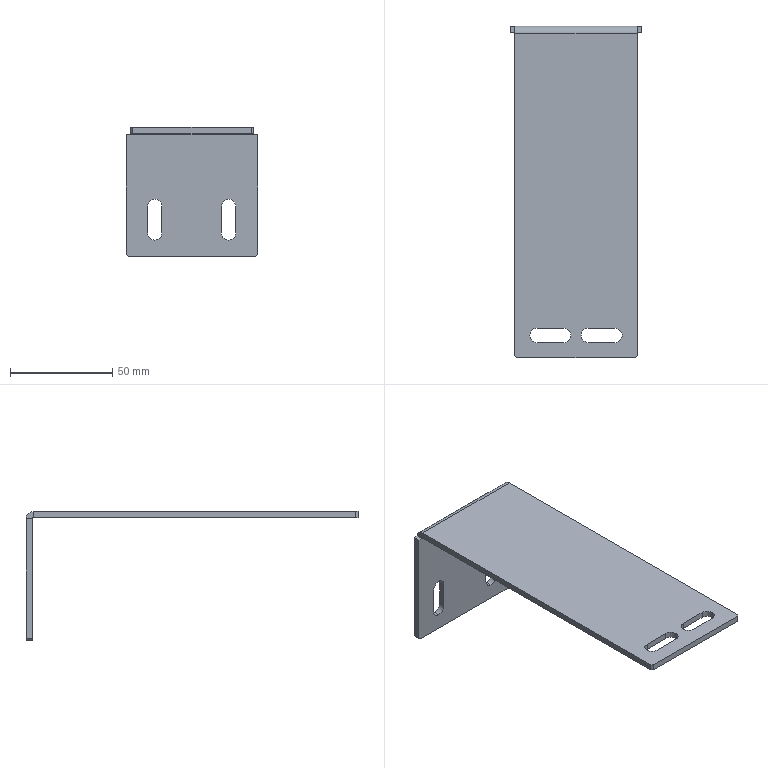Part | SolidWorks | features HoleWzd 2, Chamfer 1, EdgeFlange 1, FlatPattern 1, SMBaseFlange 1, SheetMetal 1 | 1 solid | 40 faces | box 64 x 162 x 63 mm | volume 38960 mm3 | plane 26 | cylinder 14 | commonest cylinder face diameters 7 x13 1 x1
STEP:
#1=CARTESIAN_POINT('',(17.85,81.,-55.));
#2=VERTEX_POINT('',#1);
#3=CARTESIAN_POINT('',(21.35,81.,-51.5));
#4=VERTEX_POINT('',#3);
#5=CARTESIAN_POINT('',(17.85,81.,-51.5));
#6=DIRECTION('',(0.,-1.,0.));
#7=DIRECTION('',(0.,0.,-1.));
#8=AXIS2_PLACEMENT_3D('',#5,#6,#7);
#9=CIRCLE('',#8,3.5);
#10=EDGE_CURVE('',#2,#4,#9,.T.);
#11=ORIENTED_EDGE('',*,*,#10,.F.);
#12=CARTESIAN_POINT('',(17.85,78.,-55.));
#13=VERTEX_POINT('',#12);
#14=CARTESIAN_POINT('',(17.85,78.,-55.));
#15=DIRECTION('',(0.,-1.,0.));
#16=VECTOR('',#15,1000.);
#17=LINE('',#14,#16);
#18=EDGE_CURVE('',#2,#13,#17,.T.);
#19=ORIENTED_EDGE('',*,*,#18,.T.);
#20=CARTESIAN_POINT('',(21.35,78.,-51.5));
#21=VERTEX_POINT('',#20);
#22=CARTESIAN_POINT('',(17.85,78.,-51.5));
#23=DIRECTION('',(0.,-1.,0.));
#24=DIRECTION('',(0.,0.,-1.));
#25=AXIS2_PLACEMENT_3D('',#22,#23,#24);
#26=CIRCLE('',#25,3.5);
#27=EDGE_CURVE('',#13,#21,#26,.T.);
#28=ORIENTED_EDGE('',*,*,#27,.T.);
#29=CARTESIAN_POINT('',(21.35,81.,-51.5));
#30=DIRECTION('',(0.,1.,0.));
#31=VECTOR('',#30,1000.);
#32=LINE('',#29,#31);
#33=EDGE_CURVE('',#21,#4,#32,.T.);
#34=ORIENTED_EDGE('',*,*,#33,.T.);
#35=EDGE_LOOP('',(#11,#19,#28,#34));
#36=FACE_OUTER_BOUND('',#35,.T.);
#37=CARTESIAN_POINT('',(17.85,78.,-51.5));
#38=DIRECTION('',(0.,-1.,0.));
#39=DIRECTION('',(0.,0.,-1.));
#40=AXIS2_PLACEMENT_3D('',#37,#38,#39);
#41=CYLINDRICAL_SURFACE('',#40,3.5);
#42=ADVANCED_FACE('',(#36),#41,.F.);
#43=CARTESIAN_POINT('',(-18.15,81.,-55.));
#44=VERTEX_POINT('',#43);
#45=CARTESIAN_POINT('',(-14.65,81.,-51.5));
#46=VERTEX_POINT('',#45);
#47=CARTESIAN_POINT('',(-18.15,81.,-51.5));
#48=DIRECTION('',(0.,-1.,0.));
#49=DIRECTION('',(0.,0.,-1.));
#50=AXIS2_PLACEMENT_3D('',#47,#48,#49);
#51=CIRCLE('',#50,3.5);
#52=EDGE_CURVE('',#44,#46,#51,.T.);
#53=ORIENTED_EDGE('',*,*,#52,.F.);
#54=CARTESIAN_POINT('',(-18.15,78.,-55.));
#55=VERTEX_POINT('',#54);
#56=CARTESIAN_POINT('',(-18.15,78.,-55.));
#57=DIRECTION('',(0.,-1.,0.));
#58=VECTOR('',#57,1000.);
#59=LINE('',#56,#58);
#60=EDGE_CURVE('',#44,#55,#59,.T.);
#61=ORIENTED_EDGE('',*,*,#60,.T.);
#62=CARTESIAN_POINT('',(-14.65,78.,-51.5));
#63=VERTEX_POINT('',#62);
#64=CARTESIAN_POINT('',(-18.15,78.,-51.5));
#65=DIRECTION('',(0.,-1.,0.));
#66=DIRECTION('',(0.,0.,-1.));
#67=AXIS2_PLACEMENT_3D('',#64,#65,#66);
#68=CIRCLE('',#67,3.5);
#69=EDGE_CURVE('',#55,#63,#68,.T.);
#70=ORIENTED_EDGE('',*,*,#69,.T.);
#71=CARTESIAN_POINT('',(-14.65,81.,-51.5));
#72=DIRECTION('',(0.,1.,0.));
#73=VECTOR('',#72,1000.);
#74=LINE('',#71,#73);
#75=EDGE_CURVE('',#63,#46,#74,.T.);
#76=ORIENTED_EDGE('',*,*,#75,.T.);
#77=EDGE_LOOP('',(#53,#61,#70,#76));
#78=FACE_OUTER_BOUND('',#77,.T.);
#79=CARTESIAN_POINT('',(-18.15,78.,-51.5));
#80=DIRECTION('',(0.,-1.,0.));
#81=DIRECTION('',(0.,0.,-1.));
#82=AXIS2_PLACEMENT_3D('',#79,#80,#81);
#83=CYLINDRICAL_SURFACE('',#82,3.5);
#84=ADVANCED_FACE('',(#78),#83,.F.);
#85=CARTESIAN_POINT('',(2.5,-70.,0.));
#86=VERTEX_POINT('',#85);
#87=CARTESIAN_POINT('',(6.,-66.5,0.));
#88=VERTEX_POINT('',#87);
#89=CARTESIAN_POINT('',(6.,-70.,0.));
#90=DIRECTION('',(0.,0.,-1.));
#91=DIRECTION('',(-1.,0.,0.));
#92=AXIS2_PLACEMENT_3D('',#89,#90,#91);
#93=CIRCLE('',#92,3.5);
#94=EDGE_CURVE('',#86,#88,#93,.T.);
#95=ORIENTED_EDGE('',*,*,#94,.F.);
#96=CARTESIAN_POINT('',(2.5,-70.,-3.));
#97=VERTEX_POINT('',#96);
#98=CARTESIAN_POINT('',(2.5,-70.,-3.));
#99=DIRECTION('',(0.,0.,-1.));
#100=VECTOR('',#99,1000.);
#101=LINE('',#98,#100);
#102=EDGE_CURVE('',#86,#97,#101,.T.);
#103=ORIENTED_EDGE('',*,*,#102,.T.);
#104=CARTESIAN_POINT('',(6.,-66.5,-3.));
#105=VERTEX_POINT('',#104);
#106=CARTESIAN_POINT('',(6.,-70.,-3.));
#107=DIRECTION('',(0.,0.,-1.));
#108=DIRECTION('',(-1.,0.,0.));
#109=AXIS2_PLACEMENT_3D('',#106,#107,#108);
#110=CIRCLE('',#109,3.5);
#111=EDGE_CURVE('',#97,#105,#110,.T.);
#112=ORIENTED_EDGE('',*,*,#111,.T.);
#113=CARTESIAN_POINT('',(6.,-66.5,-3.));
#114=DIRECTION('',(0.,0.,-1.));
#115=VECTOR('',#114,1000.);
#116=LINE('',#113,#115);
#117=EDGE_CURVE('',#88,#105,#116,.T.);
#118=ORIENTED_EDGE('',*,*,#117,.F.);
#119=EDGE_LOOP('',(#95,#103,#112,#118));
#120=FACE_OUTER_BOUND('',#119,.T.);
#121=CARTESIAN_POINT('',(6.,-70.,-3.));
#122=DIRECTION('',(0.,0.,-1.));
#123=DIRECTION('',(-1.,0.,0.));
#124=AXIS2_PLACEMENT_3D('',#121,#122,#123);
#125=CYLINDRICAL_SURFACE('',#124,3.5);
#126=ADVANCED_FACE('',(#120),#125,.F.);
#127=CARTESIAN_POINT('',(-22.5,-70.,0.));
#128=VERTEX_POINT('',#127);
#129=CARTESIAN_POINT('',(-19.,-66.5,0.));
#130=VERTEX_POINT('',#129);
#131=CARTESIAN_POINT('',(-19.,-70.,0.));
#132=DIRECTION('',(0.,0.,-1.));
#133=DIRECTION('',(-1.,0.,0.));
#134=AXIS2_PLACEMENT_3D('',#131,#132,#133);
#135=CIRCLE('',#134,3.5);
#136=EDGE_CURVE('',#128,#130,#135,.T.);
#137=ORIENTED_EDGE('',*,*,#136,.F.);
#138=CARTESIAN_POINT('',(-22.5,-70.,-3.));
#139=VERTEX_POINT('',#138);
#140=CARTESIAN_POINT('',(-22.5,-70.,-3.));
#141=DIRECTION('',(0.,0.,-1.));
#142=VECTOR('',#141,1000.);
#143=LINE('',#140,#142);
#144=EDGE_CURVE('',#128,#139,#143,.T.);
#145=ORIENTED_EDGE('',*,*,#144,.T.);
#146=CARTESIAN_POINT('',(-19.,-66.5,-3.));
#147=VERTEX_POINT('',#146);
#148=CARTESIAN_POINT('',(-19.,-70.,-3.));
#149=DIRECTION('',(0.,0.,-1.));
#150=DIRECTION('',(-1.,0.,0.));
#151=AXIS2_PLACEMENT_3D('',#148,#149,#150);
#152=CIRCLE('',#151,3.5);
#153=EDGE_CURVE('',#139,#147,#152,.T.);
#154=ORIENTED_EDGE('',*,*,#153,.T.);
#155=CARTESIAN_POINT('',(-19.,-66.5,-3.));
#156=DIRECTION('',(0.,0.,-1.));
#157=VECTOR('',#156,1000.);
#158=LINE('',#155,#157);
#159=EDGE_CURVE('',#130,#147,#158,.T.);
#160=ORIENTED_EDGE('',*,*,#159,.F.);
#161=EDGE_LOOP('',(#137,#145,#154,#160));
#162=FACE_OUTER_BOUND('',#161,.T.);
#163=CARTESIAN_POINT('',(-19.,-70.,-3.));
#164=DIRECTION('',(0.,0.,-1.));
#165=DIRECTION('',(-1.,0.,0.));
#166=AXIS2_PLACEMENT_3D('',#163,#164,#165);
#167=CYLINDRICAL_SURFACE('',#166,3.5);
#168=ADVANCED_FACE('',(#162),#167,.F.);
#169=CARTESIAN_POINT('',(-21.65,81.,-51.5));
#170=VERTEX_POINT('',#169);
#171=CARTESIAN_POINT('',(-18.15,81.,-51.5));
#172=DIRECTION('',(0.,-1.,0.));
#173=DIRECTION('',(0.,0.,-1.));
#174=AXIS2_PLACEMENT_3D('',#171,#172,#173);
#175=CIRCLE('',#174,3.5);
#176=EDGE_CURVE('',#170,#44,#175,.T.);
#177=ORIENTED_EDGE('',*,*,#176,.T.);
#178=ORIENTED_EDGE('',*,*,#52,.T.);
#179=CARTESIAN_POINT('',(-14.65,81.,-38.5));
#180=VERTEX_POINT('',#179);
#181=CARTESIAN_POINT('',(-14.65,81.,-38.5));
#182=DIRECTION('',(0.,0.,-1.));
#183=VECTOR('',#182,1000.);
#184=LINE('',#181,#183);
#185=EDGE_CURVE('',#180,#46,#184,.T.);
#186=ORIENTED_EDGE('',*,*,#185,.F.);
#187=CARTESIAN_POINT('',(-21.65,81.,-38.5));
#188=VERTEX_POINT('',#187);
#189=CARTESIAN_POINT('',(-18.15,81.,-38.5));
#190=DIRECTION('',(0.,-1.,0.));
#191=DIRECTION('',(0.,0.,-1.));
#192=AXIS2_PLACEMENT_3D('',#189,#190,#191);
#193=CIRCLE('',#192,3.5);
#194=EDGE_CURVE('',#180,#188,#193,.T.);
#195=ORIENTED_EDGE('',*,*,#194,.T.);
#196=CARTESIAN_POINT('',(-21.65,81.,-38.5));
#197=DIRECTION('',(0.,0.,-1.));
#198=VECTOR('',#197,1000.);
#199=LINE('',#196,#198);
#200=EDGE_CURVE('',#188,#170,#199,.T.);
#201=ORIENTED_EDGE('',*,*,#200,.T.);
#202=EDGE_LOOP('',(#177,#178,#186,#195,#201));
#203=FACE_BOUND('',#202,.T.);
#204=CARTESIAN_POINT('',(-31.,81.,-63.));
#205=VERTEX_POINT('',#204);
#206=CARTESIAN_POINT('',(31.,81.,-63.));
#207=VERTEX_POINT('',#206);
#208=CARTESIAN_POINT('',(32.,81.,-63.));
#209=DIRECTION('',(1.,0.,0.));
#210=VECTOR('',#209,1000.);
#211=LINE('',#208,#210);
#212=EDGE_CURVE('',#205,#207,#211,.T.);
#213=ORIENTED_EDGE('',*,*,#212,.F.);
#214=CARTESIAN_POINT('',(-32.,81.,-62.));
#215=VERTEX_POINT('',#214);
#216=CARTESIAN_POINT('',(-47.,81.,-47.));
#217=DIRECTION('',(-0.7071,0.,0.7071));
#218=VECTOR('',#217,1000.);
#219=LINE('',#216,#218);
#220=EDGE_CURVE('',#205,#215,#219,.T.);
#221=ORIENTED_EDGE('',*,*,#220,.T.);
#222=CARTESIAN_POINT('',(-32.,81.,-3.5));
#223=VERTEX_POINT('',#222);
#224=CARTESIAN_POINT('',(-32.,81.,-3.));
#225=DIRECTION('',(0.,0.,-1.));
#226=VECTOR('',#225,1000.);
#227=LINE('',#224,#226);
#228=EDGE_CURVE('',#223,#215,#227,.T.);
#229=ORIENTED_EDGE('',*,*,#228,.F.);
#230=CARTESIAN_POINT('',(-30.,81.,-3.5));
#231=VERTEX_POINT('',#230);
#232=CARTESIAN_POINT('',(0.,81.,-3.5));
#233=DIRECTION('',(1.,0.,0.));
#234=VECTOR('',#233,1000.);
#235=LINE('',#232,#234);
#236=EDGE_CURVE('',#223,#231,#235,.T.);
#237=ORIENTED_EDGE('',*,*,#236,.T.);
#238=CARTESIAN_POINT('',(30.,81.,-3.5));
#239=VERTEX_POINT('',#238);
#240=CARTESIAN_POINT('',(30.,81.,-3.5));
#241=DIRECTION('',(1.,0.,0.));
#242=VECTOR('',#241,1000.);
#243=LINE('',#240,#242);
#244=EDGE_CURVE('',#231,#239,#243,.T.);
#245=ORIENTED_EDGE('',*,*,#244,.T.);
#246=CARTESIAN_POINT('',(32.,81.,-3.5));
#247=VERTEX_POINT('',#246);
#248=CARTESIAN_POINT('',(0.,81.,-3.5));
#249=DIRECTION('',(1.,0.,0.));
#250=VECTOR('',#249,1000.);
#251=LINE('',#248,#250);
#252=EDGE_CURVE('',#239,#247,#251,.T.);
#253=ORIENTED_EDGE('',*,*,#252,.T.);
#254=CARTESIAN_POINT('',(32.,81.,-62.));
#255=VERTEX_POINT('',#254);
#256=CARTESIAN_POINT('',(32.,81.,-63.));
#257=DIRECTION('',(0.,0.,1.));
#258=VECTOR('',#257,1000.);
#259=LINE('',#256,#258);
#260=EDGE_CURVE('',#255,#247,#259,.T.);
#261=ORIENTED_EDGE('',*,*,#260,.F.);
#262=CARTESIAN_POINT('',(47.,81.,-47.));
#263=DIRECTION('',(-0.7071,0.,-0.7071));
#264=VECTOR('',#263,1000.);
#265=LINE('',#262,#264);
#266=EDGE_CURVE('',#255,#207,#265,.T.);
#267=ORIENTED_EDGE('',*,*,#266,.T.);
#268=EDGE_LOOP('',(#213,#221,#229,#237,#245,#253,#261,#267));
#269=FACE_OUTER_BOUND('',#268,.T.);
#270=CARTESIAN_POINT('',(14.35,81.,-38.5));
#271=VERTEX_POINT('',#270);
#272=CARTESIAN_POINT('',(14.35,81.,-51.5));
#273=VERTEX_POINT('',#272);
#274=CARTESIAN_POINT('',(14.35,81.,-38.5));
#275=DIRECTION('',(0.,0.,-1.));
#276=VECTOR('',#275,1000.);
#277=LINE('',#274,#276);
#278=EDGE_CURVE('',#271,#273,#277,.T.);
#279=ORIENTED_EDGE('',*,*,#278,.T.);
#280=CARTESIAN_POINT('',(17.85,81.,-51.5));
#281=DIRECTION('',(0.,-1.,0.));
#282=DIRECTION('',(0.,0.,-1.));
#283=AXIS2_PLACEMENT_3D('',#280,#281,#282);
#284=CIRCLE('',#283,3.5);
#285=EDGE_CURVE('',#273,#2,#284,.T.);
#286=ORIENTED_EDGE('',*,*,#285,.T.);
#287=ORIENTED_EDGE('',*,*,#10,.T.);
#288=CARTESIAN_POINT('',(21.35,81.,-38.5));
#289=VERTEX_POINT('',#288);
#290=CARTESIAN_POINT('',(21.35,81.,-38.5));
#291=DIRECTION('',(0.,0.,-1.));
#292=VECTOR('',#291,1000.);
#293=LINE('',#290,#292);
#294=EDGE_CURVE('',#289,#4,#293,.T.);
#295=ORIENTED_EDGE('',*,*,#294,.F.);
#296=CARTESIAN_POINT('',(17.85,81.,-38.5));
#297=DIRECTION('',(0.,-1.,0.));
#298=DIRECTION('',(0.,0.,-1.));
#299=AXIS2_PLACEMENT_3D('',#296,#297,#298);
#300=CIRCLE('',#299,3.5);
#301=EDGE_CURVE('',#289,#271,#300,.T.);
#302=ORIENTED_EDGE('',*,*,#301,.T.);
#303=EDGE_LOOP('',(#279,#286,#287,#295,#302));
#304=FACE_BOUND('',#303,.T.);
#305=CARTESIAN_POINT('',(0.,81.,0.));
#306=DIRECTION('',(0.,1.,0.));
#307=DIRECTION('',(0.,0.,1.));
#308=AXIS2_PLACEMENT_3D('',#305,#306,#307);
#309=PLANE('',#308);
#310=ADVANCED_FACE('',(#203,#269,#304),#309,.T.);
#311=CARTESIAN_POINT('',(21.35,78.,-38.5));
#312=VERTEX_POINT('',#311);
#313=CARTESIAN_POINT('',(14.35,78.,-38.5));
#314=VERTEX_POINT('',#313);
#315=CARTESIAN_POINT('',(17.85,78.,-38.5));
#316=DIRECTION('',(0.,-1.,0.));
#317=DIRECTION('',(0.,0.,-1.));
#318=AXIS2_PLACEMENT_3D('',#315,#316,#317);
#319=CIRCLE('',#318,3.5);
#320=EDGE_CURVE('',#312,#314,#319,.T.);
#321=ORIENTED_EDGE('',*,*,#320,.F.);
#322=CARTESIAN_POINT('',(21.35,78.,-38.5));
#323=DIRECTION('',(0.,0.,-1.));
#324=VECTOR('',#323,1000.);
#325=LINE('',#322,#324);
#326=EDGE_CURVE('',#312,#21,#325,.T.);
#327=ORIENTED_EDGE('',*,*,#326,.T.);
#328=ORIENTED_EDGE('',*,*,#27,.F.);
#329=CARTESIAN_POINT('',(14.35,78.,-51.5));
#330=VERTEX_POINT('',#329);
#331=CARTESIAN_POINT('',(17.85,78.,-51.5));
#332=DIRECTION('',(0.,-1.,0.));
#333=DIRECTION('',(0.,0.,-1.));
#334=AXIS2_PLACEMENT_3D('',#331,#332,#333);
#335=CIRCLE('',#334,3.5);
#336=EDGE_CURVE('',#330,#13,#335,.T.);
#337=ORIENTED_EDGE('',*,*,#336,.F.);
#338=CARTESIAN_POINT('',(14.35,78.,-38.5));
#339=DIRECTION('',(0.,0.,-1.));
#340=VECTOR('',#339,1000.);
#341=LINE('',#338,#340);
#342=EDGE_CURVE('',#314,#330,#341,.T.);
#343=ORIENTED_EDGE('',*,*,#342,.F.);
#344=EDGE_LOOP('',(#321,#327,#328,#337,#343));
#345=FACE_BOUND('',#344,.T.);
#346=CARTESIAN_POINT('',(-32.,78.,-3.5));
#347=VERTEX_POINT('',#346);
#348=CARTESIAN_POINT('',(-32.,78.,-62.));
#349=VERTEX_POINT('',#348);
#350=CARTESIAN_POINT('',(-32.,78.,0.));
#351=DIRECTION('',(0.,0.,-1.));
#352=VECTOR('',#351,1000.);
#353=LINE('',#350,#352);
#354=EDGE_CURVE('',#347,#349,#353,.T.);
#355=ORIENTED_EDGE('',*,*,#354,.T.);
#356=CARTESIAN_POINT('',(-31.,78.,-63.));
#357=VERTEX_POINT('',#356);
#358=CARTESIAN_POINT('',(-32.,78.,-62.));
#359=DIRECTION('',(0.7071,0.,-0.7071));
#360=VECTOR('',#359,1000.);
#361=LINE('',#358,#360);
#362=EDGE_CURVE('',#349,#357,#361,.T.);
#363=ORIENTED_EDGE('',*,*,#362,.T.);
#364=CARTESIAN_POINT('',(31.,78.,-63.));
#365=VERTEX_POINT('',#364);
#366=CARTESIAN_POINT('',(0.,78.,-63.));
#367=DIRECTION('',(1.,0.,0.));
#368=VECTOR('',#367,1000.);
#369=LINE('',#366,#368);
#370=EDGE_CURVE('',#357,#365,#369,.T.);
#371=ORIENTED_EDGE('',*,*,#370,.T.);
#372=CARTESIAN_POINT('',(32.,78.,-62.));
#373=VERTEX_POINT('',#372);
#374=CARTESIAN_POINT('',(31.,78.,-63.));
#375=DIRECTION('',(0.7071,0.,0.7071));
#376=VECTOR('',#375,1000.);
#377=LINE('',#374,#376);
#378=EDGE_CURVE('',#365,#373,#377,.T.);
#379=ORIENTED_EDGE('',*,*,#378,.T.);
#380=CARTESIAN_POINT('',(32.,78.,-3.5));
#381=VERTEX_POINT('',#380);
#382=CARTESIAN_POINT('',(32.,78.,0.));
#383=DIRECTION('',(0.,0.,1.));
#384=VECTOR('',#383,1000.);
#385=LINE('',#382,#384);
#386=EDGE_CURVE('',#373,#381,#385,.T.);
#387=ORIENTED_EDGE('',*,*,#386,.T.);
#388=CARTESIAN_POINT('',(30.,78.,-3.5));
#389=VERTEX_POINT('',#388);
#390=CARTESIAN_POINT('',(-32.,78.,-3.5));
#391=DIRECTION('',(1.,0.,0.));
#392=VECTOR('',#391,1000.);
#393=LINE('',#390,#392);
#394=EDGE_CURVE('',#389,#381,#393,.T.);
#395=ORIENTED_EDGE('',*,*,#394,.F.);
#396=CARTESIAN_POINT('',(-30.,78.,-3.5));
#397=VERTEX_POINT('',#396);
#398=CARTESIAN_POINT('',(30.,78.,-3.5));
#399=DIRECTION('',(1.,0.,0.));
#400=VECTOR('',#399,1000.);
#401=LINE('',#398,#400);
#402=EDGE_CURVE('',#397,#389,#401,.T.);
#403=ORIENTED_EDGE('',*,*,#402,.F.);
#404=CARTESIAN_POINT('',(-32.,78.,-3.5));
#405=DIRECTION('',(1.,0.,0.));
#406=VECTOR('',#405,1000.);
#407=LINE('',#404,#406);
#408=EDGE_CURVE('',#347,#397,#407,.T.);
#409=ORIENTED_EDGE('',*,*,#408,.F.);
#410=EDGE_LOOP('',(#355,#363,#371,#379,#387,#395,#403,#409));
#411=FACE_OUTER_BOUND('',#410,.T.);
#412=CARTESIAN_POINT('',(-21.65,78.,-51.5));
#413=VERTEX_POINT('',#412);
#414=CARTESIAN_POINT('',(-18.15,78.,-51.5));
#415=DIRECTION('',(0.,-1.,0.));
#416=DIRECTION('',(0.,0.,-1.));
#417=AXIS2_PLACEMENT_3D('',#414,#415,#416);
#418=CIRCLE('',#417,3.5);
#419=EDGE_CURVE('',#413,#55,#418,.T.);
#420=ORIENTED_EDGE('',*,*,#419,.F.);
#421=CARTESIAN_POINT('',(-21.65,78.,-38.5));
#422=VERTEX_POINT('',#421);
#423=CARTESIAN_POINT('',(-21.65,78.,-38.5));
#424=DIRECTION('',(0.,0.,-1.));
#425=VECTOR('',#424,1000.);
#426=LINE('',#423,#425);
#427=EDGE_CURVE('',#422,#413,#426,.T.);
#428=ORIENTED_EDGE('',*,*,#427,.F.);
#429=CARTESIAN_POINT('',(-14.65,78.,-38.5));
#430=VERTEX_POINT('',#429);
#431=CARTESIAN_POINT('',(-18.15,78.,-38.5));
#432=DIRECTION('',(0.,-1.,0.));
#433=DIRECTION('',(0.,0.,-1.));
#434=AXIS2_PLACEMENT_3D('',#431,#432,#433);
#435=CIRCLE('',#434,3.5);
#436=EDGE_CURVE('',#430,#422,#435,.T.);
#437=ORIENTED_EDGE('',*,*,#436,.F.);
#438=CARTESIAN_POINT('',(-14.65,78.,-38.5));
#439=DIRECTION('',(0.,0.,-1.));
#440=VECTOR('',#439,1000.);
#441=LINE('',#438,#440);
#442=EDGE_CURVE('',#430,#63,#441,.T.);
#443=ORIENTED_EDGE('',*,*,#442,.T.);
#444=ORIENTED_EDGE('',*,*,#69,.F.);
#445=EDGE_LOOP('',(#420,#428,#437,#443,#444));
#446=FACE_BOUND('',#445,.T.);
#447=CARTESIAN_POINT('',(0.,78.,0.));
#448=DIRECTION('',(0.,1.,0.));
#449=DIRECTION('',(0.,0.,1.));
#450=AXIS2_PLACEMENT_3D('',#447,#448,#449);
#451=PLANE('',#450);
#452=ADVANCED_FACE('',(#345,#411,#446),#451,.F.);
#453=CARTESIAN_POINT('',(30.,-80.,0.));
#454=VERTEX_POINT('',#453);
#455=CARTESIAN_POINT('',(30.,77.5,0.));
#456=VERTEX_POINT('',#455);
#457=CARTESIAN_POINT('',(30.,81.,0.));
#458=DIRECTION('',(0.,1.,0.));
#459=VECTOR('',#458,1000.);
#460=LINE('',#457,#459);
#461=EDGE_CURVE('',#454,#456,#460,.T.);
#462=ORIENTED_EDGE('',*,*,#461,.F.);
#463=CARTESIAN_POINT('',(30.,-80.,-3.));
#464=VERTEX_POINT('',#463);
#465=CARTESIAN_POINT('',(30.,-80.,-3.));
#466=DIRECTION('',(0.,0.,-1.));
#467=VECTOR('',#466,1000.);
#468=LINE('',#465,#467);
#469=EDGE_CURVE('',#454,#464,#468,.T.);
#470=ORIENTED_EDGE('',*,*,#469,.T.);
#471=CARTESIAN_POINT('',(30.,77.5,-3.));
#472=VERTEX_POINT('',#471);
#473=CARTESIAN_POINT('',(30.,81.,-3.));
#474=DIRECTION('',(0.,1.,0.));
#475=VECTOR('',#474,1000.);
#476=LINE('',#473,#475);
#477=EDGE_CURVE('',#464,#472,#476,.T.);
#478=ORIENTED_EDGE('',*,*,#477,.T.);
#479=CARTESIAN_POINT('',(30.,77.5,-3.));
#480=DIRECTION('',(0.,0.,1.));
#481=VECTOR('',#480,1000.);
#482=LINE('',#479,#481);
#483=EDGE_CURVE('',#472,#456,#482,.T.);
#484=ORIENTED_EDGE('',*,*,#483,.T.);
#485=EDGE_LOOP('',(#462,#470,#478,#484));
#486=FACE_OUTER_BOUND('',#485,.T.);
#487=CARTESIAN_POINT('',(30.,81.,-3.));
#488=DIRECTION('',(1.,0.,0.));
#489=DIRECTION('',(0.,1.,0.));
#490=AXIS2_PLACEMENT_3D('',#487,#488,#489);
#491=PLANE('',#490);
#492=ADVANCED_FACE('',(#486),#491,.T.);
#493=CARTESIAN_POINT('',(6.,-73.5,-3.));
#494=VERTEX_POINT('',#493);
#495=CARTESIAN_POINT('',(6.,-70.,-3.));
#496=DIRECTION('',(0.,0.,-1.));
#497=DIRECTION('',(-1.,0.,0.));
#498=AXIS2_PLACEMENT_3D('',#495,#496,#497);
#499=CIRCLE('',#498,3.5);
#500=EDGE_CURVE('',#494,#97,#499,.T.);
#501=ORIENTED_EDGE('',*,*,#500,.F.);
#502=CARTESIAN_POINT('',(19.,-73.5,-3.));
#503=VERTEX_POINT('',#502);
#504=CARTESIAN_POINT('',(6.,-73.5,-3.));
#505=DIRECTION('',(1.,0.,0.));
#506=VECTOR('',#505,1000.);
#507=LINE('',#504,#506);
#508=EDGE_CURVE('',#494,#503,#507,.T.);
#509=ORIENTED_EDGE('',*,*,#508,.T.);
#510=CARTESIAN_POINT('',(19.,-66.5,-3.));
#511=VERTEX_POINT('',#510);
#512=CARTESIAN_POINT('',(19.,-70.,-3.));
#513=DIRECTION('',(0.,0.,-1.));
#514=DIRECTION('',(-1.,0.,0.));
#515=AXIS2_PLACEMENT_3D('',#512,#513,#514);
#516=CIRCLE('',#515,3.5);
#517=EDGE_CURVE('',#511,#503,#516,.T.);
#518=ORIENTED_EDGE('',*,*,#517,.F.);
#519=CARTESIAN_POINT('',(6.,-66.5,-3.));
#520=DIRECTION('',(1.,0.,0.));
#521=VECTOR('',#520,1000.);
#522=LINE('',#519,#521);
#523=EDGE_CURVE('',#105,#511,#522,.T.);
#524=ORIENTED_EDGE('',*,*,#523,.F.);
#525=ORIENTED_EDGE('',*,*,#111,.F.);
#526=EDGE_LOOP('',(#501,#509,#518,#524,#525));
#527=FACE_BOUND('',#526,.T.);
#528=CARTESIAN_POINT('',(-19.,-73.5,-3.));
#529=VERTEX_POINT('',#528);
#530=CARTESIAN_POINT('',(-19.,-70.,-3.));
#531=DIRECTION('',(0.,0.,-1.));
#532=DIRECTION('',(-1.,0.,0.));
#533=AXIS2_PLACEMENT_3D('',#530,#531,#532);
#534=CIRCLE('',#533,3.5);
#535=EDGE_CURVE('',#529,#139,#534,.T.);
#536=ORIENTED_EDGE('',*,*,#535,.F.);
#537=CARTESIAN_POINT('',(-6.,-73.5,-3.));
#538=VERTEX_POINT('',#537);
#539=CARTESIAN_POINT('',(-19.,-73.5,-3.));
#540=DIRECTION('',(1.,0.,0.));
#541=VECTOR('',#540,1000.);
#542=LINE('',#539,#541);
#543=EDGE_CURVE('',#529,#538,#542,.T.);
#544=ORIENTED_EDGE('',*,*,#543,.T.);
#545=CARTESIAN_POINT('',(-6.,-66.5,-3.));
#546=VERTEX_POINT('',#545);
#547=CARTESIAN_POINT('',(-6.,-70.,-3.));
#548=DIRECTION('',(0.,0.,-1.));
#549=DIRECTION('',(-1.,0.,0.));
#550=AXIS2_PLACEMENT_3D('',#547,#548,#549);
#551=CIRCLE('',#550,3.5);
#552=EDGE_CURVE('',#546,#538,#551,.T.);
#553=ORIENTED_EDGE('',*,*,#552,.F.);
#554=CARTESIAN_POINT('',(-19.,-66.5,-3.));
#555=DIRECTION('',(1.,0.,0.));
#556=VECTOR('',#555,1000.);
#557=LINE('',#554,#556);
#558=EDGE_CURVE('',#147,#546,#557,.T.);
#559=ORIENTED_EDGE('',*,*,#558,.F.);
#560=ORIENTED_EDGE('',*,*,#153,.F.);
#561=EDGE_LOOP('',(#536,#544,#553,#559,#560));
#562=FACE_BOUND('',#561,.T.);
#563=ORIENTED_EDGE('',*,*,#477,.F.);
#564=CARTESIAN_POINT('',(29.,-81.,-3.));
#565=VERTEX_POINT('',#564);
#566=CARTESIAN_POINT('',(29.,-81.,-3.));
#567=DIRECTION('',(-0.7071,-0.7071,0.));
#568=VECTOR('',#567,1000.);
#569=LINE('',#566,#568);
#570=EDGE_CURVE('',#464,#565,#569,.T.);
#571=ORIENTED_EDGE('',*,*,#570,.T.);
#572=CARTESIAN_POINT('',(-29.,-81.,-3.));
#573=VERTEX_POINT('',#572);
#574=CARTESIAN_POINT('',(-30.,-81.,-3.));
#575=DIRECTION('',(1.,0.,0.));
#576=VECTOR('',#575,1000.);
#577=LINE('',#574,#576);
#578=EDGE_CURVE('',#573,#565,#577,.T.);
#579=ORIENTED_EDGE('',*,*,#578,.F.);
#580=CARTESIAN_POINT('',(-30.,-80.,-3.));
#581=VERTEX_POINT('',#580);
#582=CARTESIAN_POINT('',(-30.,-80.,-3.));
#583=DIRECTION('',(-0.7071,0.7071,0.));
#584=VECTOR('',#583,1000.);
#585=LINE('',#582,#584);
#586=EDGE_CURVE('',#573,#581,#585,.T.);
#587=ORIENTED_EDGE('',*,*,#586,.T.);
#588=CARTESIAN_POINT('',(-30.,77.5,-3.));
#589=VERTEX_POINT('',#588);
#590=CARTESIAN_POINT('',(-30.,81.,-3.));
#591=DIRECTION('',(0.,-1.,0.));
#592=VECTOR('',#591,1000.);
#593=LINE('',#590,#592);
#594=EDGE_CURVE('',#589,#581,#593,.T.);
#595=ORIENTED_EDGE('',*,*,#594,.F.);
#596=CARTESIAN_POINT('',(30.,77.5,-3.));
#597=DIRECTION('',(-1.,0.,0.));
#598=VECTOR('',#597,1000.);
#599=LINE('',#596,#598);
#600=EDGE_CURVE('',#472,#589,#599,.T.);
#601=ORIENTED_EDGE('',*,*,#600,.F.);
#602=EDGE_LOOP('',(#563,#571,#579,#587,#595,#601));
#603=FACE_OUTER_BOUND('',#602,.T.);
#604=CARTESIAN_POINT('',(0.,0.,-3.));
#605=DIRECTION('',(0.,0.,1.));
#606=DIRECTION('',(1.,0.,0.));
#607=AXIS2_PLACEMENT_3D('',#604,#605,#606);
#608=PLANE('',#607);
#609=ADVANCED_FACE('',(#527,#562,#603),#608,.F.);
#610=CARTESIAN_POINT('',(6.,-73.5,0.));
#611=VERTEX_POINT('',#610);
#612=CARTESIAN_POINT('',(19.,-73.5,0.));
#613=VERTEX_POINT('',#612);
#614=CARTESIAN_POINT('',(6.,-73.5,0.));
#615=DIRECTION('',(1.,0.,0.));
#616=VECTOR('',#615,1000.);
#617=LINE('',#614,#616);
#618=EDGE_CURVE('',#611,#613,#617,.T.);
#619=ORIENTED_EDGE('',*,*,#618,.F.);
#620=CARTESIAN_POINT('',(6.,-70.,0.));
#621=DIRECTION('',(0.,0.,-1.));
#622=DIRECTION('',(-1.,0.,0.));
#623=AXIS2_PLACEMENT_3D('',#620,#621,#622);
#624=CIRCLE('',#623,3.5);
#625=EDGE_CURVE('',#611,#86,#624,.T.);
#626=ORIENTED_EDGE('',*,*,#625,.T.);
#627=ORIENTED_EDGE('',*,*,#94,.T.);
#628=CARTESIAN_POINT('',(19.,-66.5,0.));
#629=VERTEX_POINT('',#628);
#630=CARTESIAN_POINT('',(6.,-66.5,0.));
#631=DIRECTION('',(1.,0.,0.));
#632=VECTOR('',#631,1000.);
#633=LINE('',#630,#632);
#634=EDGE_CURVE('',#88,#629,#633,.T.);
#635=ORIENTED_EDGE('',*,*,#634,.T.);
#636=CARTESIAN_POINT('',(19.,-70.,0.));
#637=DIRECTION('',(0.,0.,-1.));
#638=DIRECTION('',(-1.,0.,0.));
#639=AXIS2_PLACEMENT_3D('',#636,#637,#638);
#640=CIRCLE('',#639,3.5);
#641=EDGE_CURVE('',#629,#613,#640,.T.);
#642=ORIENTED_EDGE('',*,*,#641,.T.);
#643=EDGE_LOOP('',(#619,#626,#627,#635,#642));
#644=FACE_BOUND('',#643,.T.);
#645=CARTESIAN_POINT('',(-6.,-66.5,0.));
#646=VERTEX_POINT('',#645);
#647=CARTESIAN_POINT('',(-19.,-66.5,0.));
#648=DIRECTION('',(1.,0.,0.));
#649=VECTOR('',#648,1000.);
#650=LINE('',#647,#649);
#651=EDGE_CURVE('',#130,#646,#650,.T.);
#652=ORIENTED_EDGE('',*,*,#651,.T.);
#653=CARTESIAN_POINT('',(-6.,-73.5,0.));
#654=VERTEX_POINT('',#653);
#655=CARTESIAN_POINT('',(-6.,-70.,0.));
#656=DIRECTION('',(0.,0.,-1.));
#657=DIRECTION('',(-1.,0.,0.));
#658=AXIS2_PLACEMENT_3D('',#655,#656,#657);
#659=CIRCLE('',#658,3.5);
#660=EDGE_CURVE('',#646,#654,#659,.T.);
#661=ORIENTED_EDGE('',*,*,#660,.T.);
#662=CARTESIAN_POINT('',(-19.,-73.5,0.));
#663=VERTEX_POINT('',#662);
#664=CARTESIAN_POINT('',(-19.,-73.5,0.));
#665=DIRECTION('',(1.,0.,0.));
#666=VECTOR('',#665,1000.);
#667=LINE('',#664,#666);
#668=EDGE_CURVE('',#663,#654,#667,.T.);
#669=ORIENTED_EDGE('',*,*,#668,.F.);
#670=CARTESIAN_POINT('',(-19.,-70.,0.));
#671=DIRECTION('',(0.,0.,-1.));
#672=DIRECTION('',(-1.,0.,0.));
#673=AXIS2_PLACEMENT_3D('',#670,#671,#672);
#674=CIRCLE('',#673,3.5);
#675=EDGE_CURVE('',#663,#128,#674,.T.);
#676=ORIENTED_EDGE('',*,*,#675,.T.);
#677=ORIENTED_EDGE('',*,*,#136,.T.);
#678=EDGE_LOOP('',(#652,#661,#669,#676,#677));
#679=FACE_BOUND('',#678,.T.);
#680=CARTESIAN_POINT('',(-29.,-81.,0.));
#681=VERTEX_POINT('',#680);
#682=CARTESIAN_POINT('',(29.,-81.,0.));
#683=VERTEX_POINT('',#682);
#684=CARTESIAN_POINT('',(-30.,-81.,0.));
#685=DIRECTION('',(1.,0.,0.));
#686=VECTOR('',#685,1000.);
#687=LINE('',#684,#686);
#688=EDGE_CURVE('',#681,#683,#687,.T.);
#689=ORIENTED_EDGE('',*,*,#688,.T.);
#690=CARTESIAN_POINT('',(55.,-55.,0.));
#691=DIRECTION('',(0.7071,0.7071,0.));
#692=VECTOR('',#691,1000.);
#693=LINE('',#690,#692);
#694=EDGE_CURVE('',#683,#454,#693,.T.);
#695=ORIENTED_EDGE('',*,*,#694,.T.);
#696=ORIENTED_EDGE('',*,*,#461,.T.);
#697=CARTESIAN_POINT('',(-30.,77.5,0.));
#698=VERTEX_POINT('',#697);
#699=CARTESIAN_POINT('',(30.,77.5,0.));
#700=DIRECTION('',(-1.,0.,0.));
#701=VECTOR('',#700,1000.);
#702=LINE('',#699,#701);
#703=EDGE_CURVE('',#456,#698,#702,.T.);
#704=ORIENTED_EDGE('',*,*,#703,.T.);
#705=CARTESIAN_POINT('',(-30.,-80.,0.));
#706=VERTEX_POINT('',#705);
#707=CARTESIAN_POINT('',(-30.,81.,0.));
#708=DIRECTION('',(0.,-1.,0.));
#709=VECTOR('',#708,1000.);
#710=LINE('',#707,#709);
#711=EDGE_CURVE('',#698,#706,#710,.T.);
#712=ORIENTED_EDGE('',*,*,#711,.T.);
#713=CARTESIAN_POINT('',(-55.,-55.,0.));
#714=DIRECTION('',(0.7071,-0.7071,0.));
#715=VECTOR('',#714,1000.);
#716=LINE('',#713,#715);
#717=EDGE_CURVE('',#706,#681,#716,.T.);
#718=ORIENTED_EDGE('',*,*,#717,.T.);
#719=EDGE_LOOP('',(#689,#695,#696,#704,#712,#718));
#720=FACE_OUTER_BOUND('',#719,.T.);
#721=CARTESIAN_POINT('',(0.,0.,0.));
#722=DIRECTION('',(0.,0.,1.));
#723=DIRECTION('',(1.,0.,0.));
#724=AXIS2_PLACEMENT_3D('',#721,#722,#723);
#725=PLANE('',#724);
#726=ADVANCED_FACE('',(#644,#679,#720),#725,.T.);
#727=ORIENTED_EDGE('',*,*,#578,.T.);
#728=CARTESIAN_POINT('',(29.,-81.,-3.));
#729=DIRECTION('',(0.,0.,1.));
#730=VECTOR('',#729,1000.);
#731=LINE('',#728,#730);
#732=EDGE_CURVE('',#565,#683,#731,.T.);
#733=ORIENTED_EDGE('',*,*,#732,.T.);
#734=ORIENTED_EDGE('',*,*,#688,.F.);
#735=CARTESIAN_POINT('',(-29.,-81.,-3.));
#736=DIRECTION('',(0.,0.,-1.));
#737=VECTOR('',#736,1000.);
#738=LINE('',#735,#737);
#739=EDGE_CURVE('',#681,#573,#738,.T.);
#740=ORIENTED_EDGE('',*,*,#739,.T.);
#741=EDGE_LOOP('',(#727,#733,#734,#740));
#742=FACE_OUTER_BOUND('',#741,.T.);
#743=CARTESIAN_POINT('',(-30.,-81.,-3.));
#744=DIRECTION('',(0.,-1.,0.));
#745=DIRECTION('',(0.,0.,-1.));
#746=AXIS2_PLACEMENT_3D('',#743,#744,#745);
#747=PLANE('',#746);
#748=ADVANCED_FACE('',(#742),#747,.T.);
#749=ORIENTED_EDGE('',*,*,#594,.T.);
#750=CARTESIAN_POINT('',(-30.,-80.,-3.));
#751=DIRECTION('',(0.,0.,1.));
#752=VECTOR('',#751,1000.);
#753=LINE('',#750,#752);
#754=EDGE_CURVE('',#581,#706,#753,.T.);
#755=ORIENTED_EDGE('',*,*,#754,.T.);
#756=ORIENTED_EDGE('',*,*,#711,.F.);
#757=CARTESIAN_POINT('',(-30.,77.5,-3.));
#758=DIRECTION('',(0.,0.,1.));
#759=VECTOR('',#758,1000.);
#760=LINE('',#757,#759);
#761=EDGE_CURVE('',#589,#698,#760,.T.);
#762=ORIENTED_EDGE('',*,*,#761,.F.);
#763=EDGE_LOOP('',(#749,#755,#756,#762));
#764=FACE_OUTER_BOUND('',#763,.T.);
#765=CARTESIAN_POINT('',(-30.,81.,-3.));
#766=DIRECTION('',(-1.,0.,0.));
#767=DIRECTION('',(0.,-1.,0.));
#768=AXIS2_PLACEMENT_3D('',#765,#766,#767);
#769=PLANE('',#768);
#770=ADVANCED_FACE('',(#764),#769,.T.);
#771=CARTESIAN_POINT('',(-30.,78.,-3.5));
#772=DIRECTION('',(0.,1.,0.));
#773=VECTOR('',#772,1000.);
#774=LINE('',#771,#773);
#775=EDGE_CURVE('',#397,#231,#774,.T.);
#776=ORIENTED_EDGE('',*,*,#775,.F.);
#777=CARTESIAN_POINT('',(-30.,77.5,-3.5));
#778=DIRECTION('',(-1.,0.,0.));
#779=DIRECTION('',(0.,0.,-1.));
#780=AXIS2_PLACEMENT_3D('',#777,#778,#779);
#781=CIRCLE('',#780,0.5);
#782=EDGE_CURVE('',#589,#397,#781,.T.);
#783=ORIENTED_EDGE('',*,*,#782,.F.);
#784=ORIENTED_EDGE('',*,*,#761,.T.);
#785=CARTESIAN_POINT('',(-30.,77.5,-3.5));
#786=DIRECTION('',(-1.,0.,0.));
#787=DIRECTION('',(0.,0.,-1.));
#788=AXIS2_PLACEMENT_3D('',#785,#786,#787);
#789=CIRCLE('',#788,3.5);
#790=EDGE_CURVE('',#698,#231,#789,.T.);
#791=ORIENTED_EDGE('',*,*,#790,.T.);
#792=EDGE_LOOP('',(#776,#783,#784,#791));
#793=FACE_OUTER_BOUND('',#792,.T.);
#794=CARTESIAN_POINT('',(-30.,77.5,-3.5));
#795=DIRECTION('',(-1.,0.,0.));
#796=DIRECTION('',(0.,0.,1.));
#797=AXIS2_PLACEMENT_3D('',#794,#795,#796);
#798=PLANE('',#797);
#799=ADVANCED_FACE('',(#793),#798,.T.);
#800=CARTESIAN_POINT('',(30.,77.5,-3.5));
#801=DIRECTION('',(1.,0.,0.));
#802=DIRECTION('',(0.,0.,-1.));
#803=AXIS2_PLACEMENT_3D('',#800,#801,#802);
#804=CIRCLE('',#803,0.5);
#805=EDGE_CURVE('',#389,#472,#804,.T.);
#806=ORIENTED_EDGE('',*,*,#805,.F.);
#807=CARTESIAN_POINT('',(30.,78.,-3.5));
#808=DIRECTION('',(0.,1.,0.));
#809=VECTOR('',#808,1000.);
#810=LINE('',#807,#809);
#811=EDGE_CURVE('',#389,#239,#810,.T.);
#812=ORIENTED_EDGE('',*,*,#811,.T.);
#813=CARTESIAN_POINT('',(30.,77.5,-3.5));
#814=DIRECTION('',(1.,0.,0.));
#815=DIRECTION('',(0.,0.,-1.));
#816=AXIS2_PLACEMENT_3D('',#813,#814,#815);
#817=CIRCLE('',#816,3.5);
#818=EDGE_CURVE('',#239,#456,#817,.T.);
#819=ORIENTED_EDGE('',*,*,#818,.T.);
#820=ORIENTED_EDGE('',*,*,#483,.F.);
#821=EDGE_LOOP('',(#806,#812,#819,#820));
#822=FACE_OUTER_BOUND('',#821,.T.);
#823=CARTESIAN_POINT('',(30.,77.5,-3.5));
#824=DIRECTION('',(-1.,0.,0.));
#825=DIRECTION('',(0.,0.,1.));
#826=AXIS2_PLACEMENT_3D('',#823,#824,#825);
#827=PLANE('',#826);
#828=ADVANCED_FACE('',(#822),#827,.F.);
#829=ORIENTED_EDGE('',*,*,#703,.F.);
#830=ORIENTED_EDGE('',*,*,#818,.F.);
#831=ORIENTED_EDGE('',*,*,#244,.F.);
#832=ORIENTED_EDGE('',*,*,#790,.F.);
#833=EDGE_LOOP('',(#829,#830,#831,#832));
#834=FACE_OUTER_BOUND('',#833,.T.);
#835=CARTESIAN_POINT('',(30.,77.5,-3.5));
#836=DIRECTION('',(1.,0.,0.));
#837=DIRECTION('',(0.,1.,0.));
#838=AXIS2_PLACEMENT_3D('',#835,#836,#837);
#839=CYLINDRICAL_SURFACE('',#838,3.5);
#840=ADVANCED_FACE('',(#834),#839,.T.);
#841=ORIENTED_EDGE('',*,*,#600,.T.);
#842=ORIENTED_EDGE('',*,*,#782,.T.);
#843=ORIENTED_EDGE('',*,*,#402,.T.);
#844=ORIENTED_EDGE('',*,*,#805,.T.);
#845=EDGE_LOOP('',(#841,#842,#843,#844));
#846=FACE_OUTER_BOUND('',#845,.T.);
#847=CARTESIAN_POINT('',(30.,77.5,-3.5));
#848=DIRECTION('',(1.,0.,0.));
#849=DIRECTION('',(0.,1.,0.));
#850=AXIS2_PLACEMENT_3D('',#847,#848,#849);
#851=CYLINDRICAL_SURFACE('',#850,0.5);
#852=ADVANCED_FACE('',(#846),#851,.F.);
#853=ORIENTED_EDGE('',*,*,#811,.F.);
#854=ORIENTED_EDGE('',*,*,#394,.T.);
#855=CARTESIAN_POINT('',(32.,78.,-3.5));
#856=DIRECTION('',(0.,1.,0.));
#857=VECTOR('',#856,1000.);
#858=LINE('',#855,#857);
#859=EDGE_CURVE('',#381,#247,#858,.T.);
#860=ORIENTED_EDGE('',*,*,#859,.T.);
#861=ORIENTED_EDGE('',*,*,#252,.F.);
#862=EDGE_LOOP('',(#853,#854,#860,#861));
#863=FACE_OUTER_BOUND('',#862,.T.);
#864=CARTESIAN_POINT('',(-32.,78.,-3.5));
#865=DIRECTION('',(0.,0.,1.));
#866=DIRECTION('',(0.,-1.,0.));
#867=AXIS2_PLACEMENT_3D('',#864,#865,#866);
#868=PLANE('',#867);
#869=ADVANCED_FACE('',(#863),#868,.T.);
#870=ORIENTED_EDGE('',*,*,#228,.T.);
#871=CARTESIAN_POINT('',(-32.,81.,-62.));
#872=DIRECTION('',(0.,-1.,0.));
#873=VECTOR('',#872,1000.);
#874=LINE('',#871,#873);
#875=EDGE_CURVE('',#215,#349,#874,.T.);
#876=ORIENTED_EDGE('',*,*,#875,.T.);
#877=ORIENTED_EDGE('',*,*,#354,.F.);
#878=CARTESIAN_POINT('',(-32.,81.,-3.5));
#879=DIRECTION('',(0.,1.,0.));
#880=VECTOR('',#879,1000.);
#881=LINE('',#878,#880);
#882=EDGE_CURVE('',#347,#223,#881,.T.);
#883=ORIENTED_EDGE('',*,*,#882,.T.);
#884=EDGE_LOOP('',(#870,#876,#877,#883));
#885=FACE_OUTER_BOUND('',#884,.T.);
#886=CARTESIAN_POINT('',(-32.,81.,-3.));
#887=DIRECTION('',(-1.,0.,0.));
#888=DIRECTION('',(0.,0.,1.));
#889=AXIS2_PLACEMENT_3D('',#886,#887,#888);
#890=PLANE('',#889);
#891=ADVANCED_FACE('',(#885),#890,.T.);
#892=ORIENTED_EDGE('',*,*,#386,.F.);
#893=CARTESIAN_POINT('',(32.,81.,-62.));
#894=DIRECTION('',(0.,1.,0.));
#895=VECTOR('',#894,1000.);
#896=LINE('',#893,#895);
#897=EDGE_CURVE('',#373,#255,#896,.T.);
#898=ORIENTED_EDGE('',*,*,#897,.T.);
#899=ORIENTED_EDGE('',*,*,#260,.T.);
#900=ORIENTED_EDGE('',*,*,#859,.F.);
#901=EDGE_LOOP('',(#892,#898,#899,#900));
#902=FACE_OUTER_BOUND('',#901,.T.);
#903=CARTESIAN_POINT('',(32.,81.,-63.));
#904=DIRECTION('',(1.,0.,0.));
#905=DIRECTION('',(0.,0.,-1.));
#906=AXIS2_PLACEMENT_3D('',#903,#904,#905);
#907=PLANE('',#906);
#908=ADVANCED_FACE('',(#902),#907,.T.);
#909=ORIENTED_EDGE('',*,*,#370,.F.);
#910=CARTESIAN_POINT('',(-31.,81.,-63.));
#911=DIRECTION('',(0.,1.,0.));
#912=VECTOR('',#911,1000.);
#913=LINE('',#910,#912);
#914=EDGE_CURVE('',#357,#205,#913,.T.);
#915=ORIENTED_EDGE('',*,*,#914,.T.);
#916=ORIENTED_EDGE('',*,*,#212,.T.);
#917=CARTESIAN_POINT('',(31.,81.,-63.));
#918=DIRECTION('',(0.,-1.,0.));
#919=VECTOR('',#918,1000.);
#920=LINE('',#917,#919);
#921=EDGE_CURVE('',#207,#365,#920,.T.);
#922=ORIENTED_EDGE('',*,*,#921,.T.);
#923=EDGE_LOOP('',(#909,#915,#916,#922));
#924=FACE_OUTER_BOUND('',#923,.T.);
#925=CARTESIAN_POINT('',(32.,81.,-63.));
#926=DIRECTION('',(0.,0.,-1.));
#927=DIRECTION('',(0.,1.,0.));
#928=AXIS2_PLACEMENT_3D('',#925,#926,#927);
#929=PLANE('',#928);
#930=ADVANCED_FACE('',(#924),#929,.T.);
#931=ORIENTED_EDGE('',*,*,#408,.T.);
#932=ORIENTED_EDGE('',*,*,#775,.T.);
#933=ORIENTED_EDGE('',*,*,#236,.F.);
#934=ORIENTED_EDGE('',*,*,#882,.F.);
#935=EDGE_LOOP('',(#931,#932,#933,#934));
#936=FACE_OUTER_BOUND('',#935,.T.);
#937=CARTESIAN_POINT('',(-32.,78.,-3.5));
#938=DIRECTION('',(0.,0.,1.));
#939=DIRECTION('',(0.,-1.,0.));
#940=AXIS2_PLACEMENT_3D('',#937,#938,#939);
#941=PLANE('',#940);
#942=ADVANCED_FACE('',(#936),#941,.T.);
#943=ORIENTED_EDGE('',*,*,#660,.F.);
#944=CARTESIAN_POINT('',(-6.,-66.5,-3.));
#945=DIRECTION('',(0.,0.,1.));
#946=VECTOR('',#945,1000.);
#947=LINE('',#944,#946);
#948=EDGE_CURVE('',#546,#646,#947,.T.);
#949=ORIENTED_EDGE('',*,*,#948,.F.);
#950=ORIENTED_EDGE('',*,*,#552,.T.);
#951=CARTESIAN_POINT('',(-6.,-73.5,-3.));
#952=DIRECTION('',(0.,0.,-1.));
#953=VECTOR('',#952,1000.);
#954=LINE('',#951,#953);
#955=EDGE_CURVE('',#654,#538,#954,.T.);
#956=ORIENTED_EDGE('',*,*,#955,.F.);
#957=EDGE_LOOP('',(#943,#949,#950,#956));
#958=FACE_OUTER_BOUND('',#957,.T.);
#959=CARTESIAN_POINT('',(-6.,-70.,-3.));
#960=DIRECTION('',(0.,0.,-1.));
#961=DIRECTION('',(-1.,0.,0.));
#962=AXIS2_PLACEMENT_3D('',#959,#960,#961);
#963=CYLINDRICAL_SURFACE('',#962,3.5);
#964=ADVANCED_FACE('',(#958),#963,.F.);
#965=ORIENTED_EDGE('',*,*,#144,.F.);
#966=ORIENTED_EDGE('',*,*,#675,.F.);
#967=CARTESIAN_POINT('',(-19.,-73.5,-3.));
#968=DIRECTION('',(0.,0.,1.));
#969=VECTOR('',#968,1000.);
#970=LINE('',#967,#969);
#971=EDGE_CURVE('',#529,#663,#970,.T.);
#972=ORIENTED_EDGE('',*,*,#971,.F.);
#973=ORIENTED_EDGE('',*,*,#535,.T.);
#974=EDGE_LOOP('',(#965,#966,#972,#973));
#975=FACE_OUTER_BOUND('',#974,.T.);
#976=CARTESIAN_POINT('',(-19.,-70.,-3.));
#977=DIRECTION('',(0.,0.,-1.));
#978=DIRECTION('',(-1.,0.,0.));
#979=AXIS2_PLACEMENT_3D('',#976,#977,#978);
#980=CYLINDRICAL_SURFACE('',#979,3.5);
#981=ADVANCED_FACE('',(#975),#980,.F.);
#982=ORIENTED_EDGE('',*,*,#955,.T.);
#983=ORIENTED_EDGE('',*,*,#543,.F.);
#984=ORIENTED_EDGE('',*,*,#971,.T.);
#985=ORIENTED_EDGE('',*,*,#668,.T.);
#986=EDGE_LOOP('',(#982,#983,#984,#985));
#987=FACE_OUTER_BOUND('',#986,.T.);
#988=CARTESIAN_POINT('',(-19.,-73.5,-3.));
#989=DIRECTION('',(0.,-1.,0.));
#990=DIRECTION('',(0.,0.,-1.));
#991=AXIS2_PLACEMENT_3D('',#988,#989,#990);
#992=PLANE('',#991);
#993=ADVANCED_FACE('',(#987),#992,.F.);
#994=ORIENTED_EDGE('',*,*,#948,.T.);
#995=ORIENTED_EDGE('',*,*,#651,.F.);
#996=ORIENTED_EDGE('',*,*,#159,.T.);
#997=ORIENTED_EDGE('',*,*,#558,.T.);
#998=EDGE_LOOP('',(#994,#995,#996,#997));
#999=FACE_OUTER_BOUND('',#998,.T.);
#1000=CARTESIAN_POINT('',(-19.,-66.5,-3.));
#1001=DIRECTION('',(0.,1.,0.));
#1002=DIRECTION('',(0.,0.,1.));
#1003=AXIS2_PLACEMENT_3D('',#1000,#1001,#1002);
#1004=PLANE('',#1003);
#1005=ADVANCED_FACE('',(#999),#1004,.F.);
#1006=ORIENTED_EDGE('',*,*,#641,.F.);
#1007=CARTESIAN_POINT('',(19.,-66.5,-3.));
#1008=DIRECTION('',(0.,0.,1.));
#1009=VECTOR('',#1008,1000.);
#1010=LINE('',#1007,#1009);
#1011=EDGE_CURVE('',#511,#629,#1010,.T.);
#1012=ORIENTED_EDGE('',*,*,#1011,.F.);
#1013=ORIENTED_EDGE('',*,*,#517,.T.);
#1014=CARTESIAN_POINT('',(19.,-73.5,-3.));
#1015=DIRECTION('',(0.,0.,-1.));
#1016=VECTOR('',#1015,1000.);
#1017=LINE('',#1014,#1016);
#1018=EDGE_CURVE('',#613,#503,#1017,.T.);
#1019=ORIENTED_EDGE('',*,*,#1018,.F.);
#1020=EDGE_LOOP('',(#1006,#1012,#1013,#1019));
#1021=FACE_OUTER_BOUND('',#1020,.T.);
#1022=CARTESIAN_POINT('',(19.,-70.,-3.));
#1023=DIRECTION('',(0.,0.,-1.));
#1024=DIRECTION('',(-1.,0.,0.));
#1025=AXIS2_PLACEMENT_3D('',#1022,#1023,#1024);
#1026=CYLINDRICAL_SURFACE('',#1025,3.5);
#1027=ADVANCED_FACE('',(#1021),#1026,.F.);
#1028=ORIENTED_EDGE('',*,*,#102,.F.);
#1029=ORIENTED_EDGE('',*,*,#625,.F.);
#1030=CARTESIAN_POINT('',(6.,-73.5,-3.));
#1031=DIRECTION('',(0.,0.,1.));
#1032=VECTOR('',#1031,1000.);
#1033=LINE('',#1030,#1032);
#1034=EDGE_CURVE('',#494,#611,#1033,.T.);
#1035=ORIENTED_EDGE('',*,*,#1034,.F.);
#1036=ORIENTED_EDGE('',*,*,#500,.T.);
#1037=EDGE_LOOP('',(#1028,#1029,#1035,#1036));
#1038=FACE_OUTER_BOUND('',#1037,.T.);
#1039=CARTESIAN_POINT('',(6.,-70.,-3.));
#1040=DIRECTION('',(0.,0.,-1.));
#1041=DIRECTION('',(-1.,0.,0.));
#1042=AXIS2_PLACEMENT_3D('',#1039,#1040,#1041);
#1043=CYLINDRICAL_SURFACE('',#1042,3.5);
#1044=ADVANCED_FACE('',(#1038),#1043,.F.);
#1045=ORIENTED_EDGE('',*,*,#1018,.T.);
#1046=ORIENTED_EDGE('',*,*,#508,.F.);
#1047=ORIENTED_EDGE('',*,*,#1034,.T.);
#1048=ORIENTED_EDGE('',*,*,#618,.T.);
#1049=EDGE_LOOP('',(#1045,#1046,#1047,#1048));
#1050=FACE_OUTER_BOUND('',#1049,.T.);
#1051=CARTESIAN_POINT('',(6.,-73.5,-3.));
#1052=DIRECTION('',(0.,-1.,0.));
#1053=DIRECTION('',(0.,0.,-1.));
#1054=AXIS2_PLACEMENT_3D('',#1051,#1052,#1053);
#1055=PLANE('',#1054);
#1056=ADVANCED_FACE('',(#1050),#1055,.F.);
#1057=ORIENTED_EDGE('',*,*,#1011,.T.);
#1058=ORIENTED_EDGE('',*,*,#634,.F.);
#1059=ORIENTED_EDGE('',*,*,#117,.T.);
#1060=ORIENTED_EDGE('',*,*,#523,.T.);
#1061=EDGE_LOOP('',(#1057,#1058,#1059,#1060));
#1062=FACE_OUTER_BOUND('',#1061,.T.);
#1063=CARTESIAN_POINT('',(6.,-66.5,-3.));
#1064=DIRECTION('',(0.,1.,0.));
#1065=DIRECTION('',(0.,0.,1.));
#1066=AXIS2_PLACEMENT_3D('',#1063,#1064,#1065);
#1067=PLANE('',#1066);
#1068=ADVANCED_FACE('',(#1062),#1067,.F.);
#1069=ORIENTED_EDGE('',*,*,#60,.F.);
#1070=ORIENTED_EDGE('',*,*,#176,.F.);
#1071=CARTESIAN_POINT('',(-21.65,78.,-51.5));
#1072=DIRECTION('',(0.,1.,0.));
#1073=VECTOR('',#1072,1000.);
#1074=LINE('',#1071,#1073);
#1075=EDGE_CURVE('',#413,#170,#1074,.T.);
#1076=ORIENTED_EDGE('',*,*,#1075,.F.);
#1077=ORIENTED_EDGE('',*,*,#419,.T.);
#1078=EDGE_LOOP('',(#1069,#1070,#1076,#1077));
#1079=FACE_OUTER_BOUND('',#1078,.T.);
#1080=CARTESIAN_POINT('',(-18.15,78.,-51.5));
#1081=DIRECTION('',(0.,-1.,0.));
#1082=DIRECTION('',(0.,0.,-1.));
#1083=AXIS2_PLACEMENT_3D('',#1080,#1081,#1082);
#1084=CYLINDRICAL_SURFACE('',#1083,3.5);
#1085=ADVANCED_FACE('',(#1079),#1084,.F.);
#1086=ORIENTED_EDGE('',*,*,#194,.F.);
#1087=CARTESIAN_POINT('',(-14.65,81.,-38.5));
#1088=DIRECTION('',(0.,1.,0.));
#1089=VECTOR('',#1088,1000.);
#1090=LINE('',#1087,#1089);
#1091=EDGE_CURVE('',#430,#180,#1090,.T.);
#1092=ORIENTED_EDGE('',*,*,#1091,.F.);
#1093=ORIENTED_EDGE('',*,*,#436,.T.);
#1094=CARTESIAN_POINT('',(-21.65,78.,-38.5));
#1095=DIRECTION('',(0.,-1.,0.));
#1096=VECTOR('',#1095,1000.);
#1097=LINE('',#1094,#1096);
#1098=EDGE_CURVE('',#188,#422,#1097,.T.);
#1099=ORIENTED_EDGE('',*,*,#1098,.F.);
#1100=EDGE_LOOP('',(#1086,#1092,#1093,#1099));
#1101=FACE_OUTER_BOUND('',#1100,.T.);
#1102=CARTESIAN_POINT('',(-18.15,78.,-38.5));
#1103=DIRECTION('',(0.,-1.,0.));
#1104=DIRECTION('',(0.,0.,-1.));
#1105=AXIS2_PLACEMENT_3D('',#1102,#1103,#1104);
#1106=CYLINDRICAL_SURFACE('',#1105,3.5);
#1107=ADVANCED_FACE('',(#1101),#1106,.F.);
#1108=ORIENTED_EDGE('',*,*,#75,.F.);
#1109=ORIENTED_EDGE('',*,*,#442,.F.);
#1110=ORIENTED_EDGE('',*,*,#1091,.T.);
#1111=ORIENTED_EDGE('',*,*,#185,.T.);
#1112=EDGE_LOOP('',(#1108,#1109,#1110,#1111));
#1113=FACE_OUTER_BOUND('',#1112,.T.);
#1114=CARTESIAN_POINT('',(-14.65,81.,-38.5));
#1115=DIRECTION('',(-1.,0.,0.));
#1116=DIRECTION('',(0.,0.,1.));
#1117=AXIS2_PLACEMENT_3D('',#1114,#1115,#1116);
#1118=PLANE('',#1117);
#1119=ADVANCED_FACE('',(#1113),#1118,.T.);
#1120=ORIENTED_EDGE('',*,*,#1075,.T.);
#1121=ORIENTED_EDGE('',*,*,#200,.F.);
#1122=ORIENTED_EDGE('',*,*,#1098,.T.);
#1123=ORIENTED_EDGE('',*,*,#427,.T.);
#1124=EDGE_LOOP('',(#1120,#1121,#1122,#1123));
#1125=FACE_OUTER_BOUND('',#1124,.T.);
#1126=CARTESIAN_POINT('',(-21.65,78.,-38.5));
#1127=DIRECTION('',(-1.,0.,0.));
#1128=DIRECTION('',(0.,0.,1.));
#1129=AXIS2_PLACEMENT_3D('',#1126,#1127,#1128);
#1130=PLANE('',#1129);
#1131=ADVANCED_FACE('',(#1125),#1130,.F.);
#1132=ORIENTED_EDGE('',*,*,#18,.F.);
#1133=ORIENTED_EDGE('',*,*,#285,.F.);
#1134=CARTESIAN_POINT('',(14.35,78.,-51.5));
#1135=DIRECTION('',(0.,1.,0.));
#1136=VECTOR('',#1135,1000.);
#1137=LINE('',#1134,#1136);
#1138=EDGE_CURVE('',#330,#273,#1137,.T.);
#1139=ORIENTED_EDGE('',*,*,#1138,.F.);
#1140=ORIENTED_EDGE('',*,*,#336,.T.);
#1141=EDGE_LOOP('',(#1132,#1133,#1139,#1140));
#1142=FACE_OUTER_BOUND('',#1141,.T.);
#1143=CARTESIAN_POINT('',(17.85,78.,-51.5));
#1144=DIRECTION('',(0.,-1.,0.));
#1145=DIRECTION('',(0.,0.,-1.));
#1146=AXIS2_PLACEMENT_3D('',#1143,#1144,#1145);
#1147=CYLINDRICAL_SURFACE('',#1146,3.5);
#1148=ADVANCED_FACE('',(#1142),#1147,.F.);
#1149=ORIENTED_EDGE('',*,*,#301,.F.);
#1150=CARTESIAN_POINT('',(21.35,81.,-38.5));
#1151=DIRECTION('',(0.,1.,0.));
#1152=VECTOR('',#1151,1000.);
#1153=LINE('',#1150,#1152);
#1154=EDGE_CURVE('',#312,#289,#1153,.T.);
#1155=ORIENTED_EDGE('',*,*,#1154,.F.);
#1156=ORIENTED_EDGE('',*,*,#320,.T.);
#1157=CARTESIAN_POINT('',(14.35,78.,-38.5));
#1158=DIRECTION('',(0.,-1.,0.));
#1159=VECTOR('',#1158,1000.);
#1160=LINE('',#1157,#1159);
#1161=EDGE_CURVE('',#271,#314,#1160,.T.);
#1162=ORIENTED_EDGE('',*,*,#1161,.F.);
#1163=EDGE_LOOP('',(#1149,#1155,#1156,#1162));
#1164=FACE_OUTER_BOUND('',#1163,.T.);
#1165=CARTESIAN_POINT('',(17.85,78.,-38.5));
#1166=DIRECTION('',(0.,-1.,0.));
#1167=DIRECTION('',(0.,0.,-1.));
#1168=AXIS2_PLACEMENT_3D('',#1165,#1166,#1167);
#1169=CYLINDRICAL_SURFACE('',#1168,3.5);
#1170=ADVANCED_FACE('',(#1164),#1169,.F.);
#1171=ORIENTED_EDGE('',*,*,#33,.F.);
#1172=ORIENTED_EDGE('',*,*,#326,.F.);
#1173=ORIENTED_EDGE('',*,*,#1154,.T.);
#1174=ORIENTED_EDGE('',*,*,#294,.T.);
#1175=EDGE_LOOP('',(#1171,#1172,#1173,#1174));
#1176=FACE_OUTER_BOUND('',#1175,.T.);
#1177=CARTESIAN_POINT('',(21.35,81.,-38.5));
#1178=DIRECTION('',(-1.,0.,0.));
#1179=DIRECTION('',(0.,0.,1.));
#1180=AXIS2_PLACEMENT_3D('',#1177,#1178,#1179);
#1181=PLANE('',#1180);
#1182=ADVANCED_FACE('',(#1176),#1181,.T.);
#1183=ORIENTED_EDGE('',*,*,#1138,.T.);
#1184=ORIENTED_EDGE('',*,*,#278,.F.);
#1185=ORIENTED_EDGE('',*,*,#1161,.T.);
#1186=ORIENTED_EDGE('',*,*,#342,.T.);
#1187=EDGE_LOOP('',(#1183,#1184,#1185,#1186));
#1188=FACE_OUTER_BOUND('',#1187,.T.);
#1189=CARTESIAN_POINT('',(14.35,78.,-38.5));
#1190=DIRECTION('',(-1.,0.,0.));
#1191=DIRECTION('',(0.,0.,1.));
#1192=AXIS2_PLACEMENT_3D('',#1189,#1190,#1191);
#1193=PLANE('',#1192);
#1194=ADVANCED_FACE('',(#1188),#1193,.F.);
#1195=ORIENTED_EDGE('',*,*,#220,.F.);
#1196=ORIENTED_EDGE('',*,*,#914,.F.);
#1197=ORIENTED_EDGE('',*,*,#362,.F.);
#1198=ORIENTED_EDGE('',*,*,#875,.F.);
#1199=EDGE_LOOP('',(#1195,#1196,#1197,#1198));
#1200=FACE_OUTER_BOUND('',#1199,.T.);
#1201=CARTESIAN_POINT('',(-32.,81.,-62.));
#1202=DIRECTION('',(0.7071,0.,0.7071));
#1203=DIRECTION('',(0.,-1.,0.));
#1204=AXIS2_PLACEMENT_3D('',#1201,#1202,#1203);
#1205=PLANE('',#1204);
#1206=ADVANCED_FACE('',(#1200),#1205,.F.);
#1207=ORIENTED_EDGE('',*,*,#266,.F.);
#1208=ORIENTED_EDGE('',*,*,#897,.F.);
#1209=ORIENTED_EDGE('',*,*,#378,.F.);
#1210=ORIENTED_EDGE('',*,*,#921,.F.);
#1211=EDGE_LOOP('',(#1207,#1208,#1209,#1210));
#1212=FACE_OUTER_BOUND('',#1211,.T.);
#1213=CARTESIAN_POINT('',(31.,81.,-63.));
#1214=DIRECTION('',(-0.7071,0.,0.7071));
#1215=DIRECTION('',(0.,-1.,0.));
#1216=AXIS2_PLACEMENT_3D('',#1213,#1214,#1215);
#1217=PLANE('',#1216);
#1218=ADVANCED_FACE('',(#1212),#1217,.F.);
#1219=ORIENTED_EDGE('',*,*,#570,.F.);
#1220=ORIENTED_EDGE('',*,*,#469,.F.);
#1221=ORIENTED_EDGE('',*,*,#694,.F.);
#1222=ORIENTED_EDGE('',*,*,#732,.F.);
#1223=EDGE_LOOP('',(#1219,#1220,#1221,#1222));
#1224=FACE_OUTER_BOUND('',#1223,.T.);
#1225=CARTESIAN_POINT('',(29.,-81.,-3.));
#1226=DIRECTION('',(-0.7071,0.7071,0.));
#1227=DIRECTION('',(0.,0.,1.));
#1228=AXIS2_PLACEMENT_3D('',#1225,#1226,#1227);
#1229=PLANE('',#1228);
#1230=ADVANCED_FACE('',(#1224),#1229,.F.);
#1231=ORIENTED_EDGE('',*,*,#586,.F.);
#1232=ORIENTED_EDGE('',*,*,#739,.F.);
#1233=ORIENTED_EDGE('',*,*,#717,.F.);
#1234=ORIENTED_EDGE('',*,*,#754,.F.);
#1235=EDGE_LOOP('',(#1231,#1232,#1233,#1234));
#1236=FACE_OUTER_BOUND('',#1235,.T.);
#1237=CARTESIAN_POINT('',(-30.,-80.,-3.));
#1238=DIRECTION('',(0.7071,0.7071,0.));
#1239=DIRECTION('',(0.,0.,1.));
#1240=AXIS2_PLACEMENT_3D('',#1237,#1238,#1239);
#1241=PLANE('',#1240);
#1242=ADVANCED_FACE('',(#1236),#1241,.F.);
#1243=CLOSED_SHELL('',(#42,#84,#126,#168,#310,#452,#492,#609,#726,#748,#770,#799,#828,#840,#852,#869,#891,#908,#930,#942,#964,#981,#993,#1005,#1027,#1044,#1056,#1068,#1085,#1107,#1119,#1131,#1148,#1170,#1182,#1194,#1206,#1218,#1230,#1242));
#1244=MANIFOLD_SOLID_BREP('',#1243);
#1245=CARTESIAN_POINT('',(0.,0.,0.));
#1246=DIRECTION('',(0.,0.,1.));
#1247=DIRECTION('',(1.,0.,0.));
#1248=AXIS2_PLACEMENT_3D('',#1245,#1246,#1247);
#1249=(LENGTH_UNIT()NAMED_UNIT(*)SI_UNIT(.MILLI.,.METRE.));
#1250=UNCERTAINTY_MEASURE_WITH_UNIT(LENGTH_MEASURE(0.00001),#1249,'','');
#1251=(NAMED_UNIT(*)PLANE_ANGLE_UNIT()SI_UNIT($,.RADIAN.));
#1252=(NAMED_UNIT(*)SI_UNIT($,.STERADIAN.)SOLID_ANGLE_UNIT());
#1253=(GEOMETRIC_REPRESENTATION_CONTEXT(3)GLOBAL_UNCERTAINTY_ASSIGNED_CONTEXT((#1250))GLOBAL_UNIT_ASSIGNED_CONTEXT((#1249,#1251,#1252))REPRESENTATION_CONTEXT('',''));
#1254=ADVANCED_BREP_SHAPE_REPRESENTATION('',(#1244,#1248),#1253);